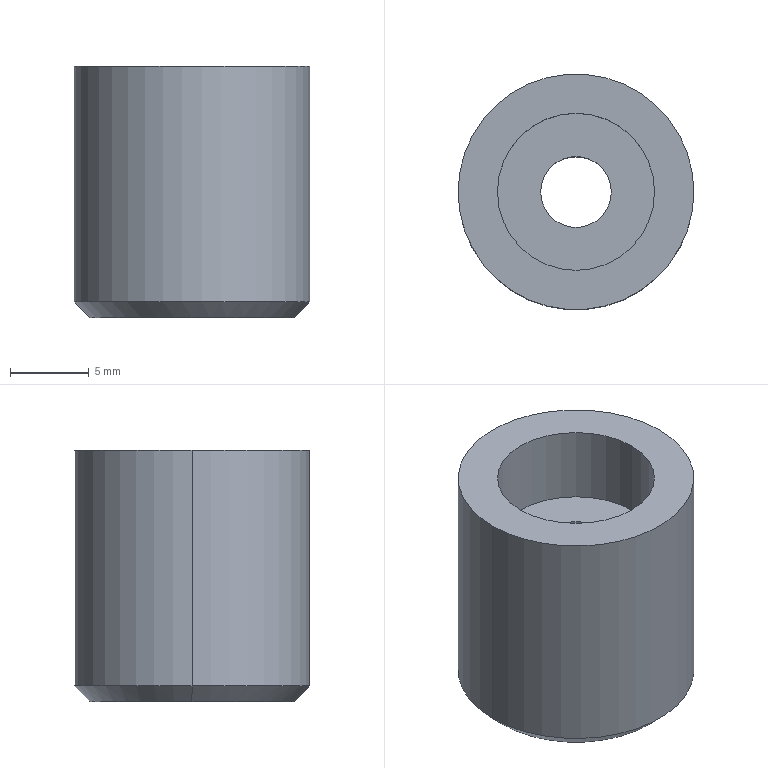Part | STEP file | 2074 Stop shaft 2 | 1 solid | 14 faces | box 15 x 15 x 16 mm | volume 2079 mm3 | cylinder 8 | plane 4 | cone 2 | commonest cylinder face diameters 4.5 x2 8 x2 10 x2 15 x2
STEP:
#1=CARTESIAN_POINT('',(0.,0.,0.));
#2=DIRECTION('',(0.,0.,1.));
#3=DIRECTION('',(1.,0.,0.));
#4=AXIS2_PLACEMENT_3D('',#1,#2,#3);
#5=CARTESIAN_POINT('',(-6.5,0.,0.));
#6=VERTEX_POINT('',#5);
#7=CARTESIAN_POINT('',(6.5,0.,0.));
#8=VERTEX_POINT('',#7);
#9=CARTESIAN_POINT('',(0.,0.,0.));
#10=DIRECTION('',(0.,0.,-1.));
#11=DIRECTION('',(1.,0.,0.));
#12=AXIS2_PLACEMENT_3D('',#9,#10,#11);
#13=CIRCLE('',#12,6.5);
#14=CARTESIAN_POINT('',(0.,0.,1.));
#15=DIRECTION('',(0.,0.,1.));
#16=DIRECTION('',(1.,0.,0.));
#17=AXIS2_PLACEMENT_3D('',#14,#15,#16);
#18=CONICAL_SURFACE('',#17,7.5,0.7854);
#19=CARTESIAN_POINT('',(6.283,-1.));
#20=DIRECTION('',(-1.,0.));
#21=VECTOR('',#20,1.);
#22=LINE('',#19,#21);
#23=(GEOMETRIC_REPRESENTATION_CONTEXT(2)PARAMETRIC_REPRESENTATION_CONTEXT()REPRESENTATION_CONTEXT('',''));
#24=DEFINITIONAL_REPRESENTATION('',(#22),#23);
#25=PCURVE('',#18,#24);
#26=CARTESIAN_POINT('',(0.,0.,0.));
#27=DIRECTION('',(0.,0.,1.));
#28=DIRECTION('',(1.,0.,0.));
#29=AXIS2_PLACEMENT_3D('',#26,#27,#28);
#30=PLANE('',#29);
#31=CARTESIAN_POINT('',(6.5,0.));
#32=CARTESIAN_POINT('',(6.5,-11.258));
#33=CARTESIAN_POINT('',(-3.25,-5.629));
#34=CARTESIAN_POINT('',(-13.,0.));
#35=CARTESIAN_POINT('',(-3.25,5.629));
#36=CARTESIAN_POINT('',(6.5,11.258));
#37=CARTESIAN_POINT('',(6.5,0.));
#38=(BOUNDED_CURVE()B_SPLINE_CURVE(2,(#31,#32,#33,#34,#35,#36,#37),.UNSPECIFIED.,.T.,.F.)B_SPLINE_CURVE_WITH_KNOTS((1,2,2,2,2,1),(-2.094,0.,2.094,4.189,6.283,8.378),.UNSPECIFIED.)CURVE()GEOMETRIC_REPRESENTATION_ITEM()RATIONAL_B_SPLINE_CURVE((1.,0.5,1.,0.5,1.,0.5,1.))REPRESENTATION_ITEM(''));
#39=(GEOMETRIC_REPRESENTATION_CONTEXT(2)PARAMETRIC_REPRESENTATION_CONTEXT()REPRESENTATION_CONTEXT('',''));
#40=DEFINITIONAL_REPRESENTATION('',(#38),#39);
#41=PCURVE('',#30,#40);
#42=SURFACE_CURVE('',#13,(#25,#41),.PCURVE_S1.);
#43=EDGE_CURVE('',#6,#8,#42,.T.);
#44=ORIENTED_EDGE('',*,*,#43,.F.);
#45=CARTESIAN_POINT('',(-7.5,0.,1.));
#46=VERTEX_POINT('',#45);
#47=CARTESIAN_POINT('',(-7.5,0.,1.));
#48=DIRECTION('',(-0.7071,0.,0.7071));
#49=VECTOR('',#48,1.);
#50=LINE('',#47,#49);
#51=CARTESIAN_POINT('',(3.142,0.));
#52=DIRECTION('',(0.,1.));
#53=VECTOR('',#52,1.);
#54=LINE('',#51,#53);
#55=(GEOMETRIC_REPRESENTATION_CONTEXT(2)PARAMETRIC_REPRESENTATION_CONTEXT()REPRESENTATION_CONTEXT('',''));
#56=DEFINITIONAL_REPRESENTATION('',(#54),#55);
#57=PCURVE('',#18,#56);
#58=CARTESIAN_POINT('',(0.,0.,1.));
#59=DIRECTION('',(0.,0.,1.));
#60=DIRECTION('',(1.,0.,0.));
#61=AXIS2_PLACEMENT_3D('',#58,#59,#60);
#62=CONICAL_SURFACE('',#61,7.5,0.7854);
#63=CARTESIAN_POINT('',(3.142,0.));
#64=DIRECTION('',(0.,1.));
#65=VECTOR('',#64,1.);
#66=LINE('',#63,#65);
#67=(GEOMETRIC_REPRESENTATION_CONTEXT(2)PARAMETRIC_REPRESENTATION_CONTEXT()REPRESENTATION_CONTEXT('',''));
#68=DEFINITIONAL_REPRESENTATION('',(#66),#67);
#69=PCURVE('',#62,#68);
#70=SURFACE_CURVE('',#50,(#57,#69),.PCURVE_S1.);
#71=EDGE_CURVE('',#6,#46,#70,.T.);
#72=ORIENTED_EDGE('',*,*,#71,.T.);
#73=CARTESIAN_POINT('',(7.5,0.,1.));
#74=VERTEX_POINT('',#73);
#75=CARTESIAN_POINT('',(0.,0.,1.));
#76=DIRECTION('',(0.,0.,1.));
#77=DIRECTION('',(1.,0.,0.));
#78=AXIS2_PLACEMENT_3D('',#75,#76,#77);
#79=CIRCLE('',#78,7.5);
#80=CARTESIAN_POINT('',(0.,0.));
#81=DIRECTION('',(1.,0.));
#82=VECTOR('',#81,1.);
#83=LINE('',#80,#82);
#84=(GEOMETRIC_REPRESENTATION_CONTEXT(2)PARAMETRIC_REPRESENTATION_CONTEXT()REPRESENTATION_CONTEXT('',''));
#85=DEFINITIONAL_REPRESENTATION('',(#83),#84);
#86=PCURVE('',#18,#85);
#87=CARTESIAN_POINT('',(0.,0.,16.));
#88=DIRECTION('',(0.,0.,-1.));
#89=DIRECTION('',(-1.,0.,0.));
#90=AXIS2_PLACEMENT_3D('',#87,#88,#89);
#91=CYLINDRICAL_SURFACE('',#90,7.5);
#92=CARTESIAN_POINT('',(3.142,15.));
#93=DIRECTION('',(-1.,0.));
#94=VECTOR('',#93,1.);
#95=LINE('',#92,#94);
#96=(GEOMETRIC_REPRESENTATION_CONTEXT(2)PARAMETRIC_REPRESENTATION_CONTEXT()REPRESENTATION_CONTEXT('',''));
#97=DEFINITIONAL_REPRESENTATION('',(#95),#96);
#98=PCURVE('',#91,#97);
#99=SURFACE_CURVE('',#79,(#86,#98),.PCURVE_S1.);
#100=EDGE_CURVE('',#74,#46,#99,.T.);
#101=ORIENTED_EDGE('',*,*,#100,.F.);
#102=CARTESIAN_POINT('',(7.5,0.,1.));
#103=DIRECTION('',(0.7071,0.,0.7071));
#104=VECTOR('',#103,1.);
#105=LINE('',#102,#104);
#106=CARTESIAN_POINT('',(0.,0.));
#107=DIRECTION('',(0.,1.));
#108=VECTOR('',#107,1.);
#109=LINE('',#106,#108);
#110=(GEOMETRIC_REPRESENTATION_CONTEXT(2)PARAMETRIC_REPRESENTATION_CONTEXT()REPRESENTATION_CONTEXT('',''));
#111=DEFINITIONAL_REPRESENTATION('',(#109),#110);
#112=PCURVE('',#18,#111);
#113=CARTESIAN_POINT('',(6.283,0.));
#114=DIRECTION('',(0.,1.));
#115=VECTOR('',#114,1.);
#116=LINE('',#113,#115);
#117=(GEOMETRIC_REPRESENTATION_CONTEXT(2)PARAMETRIC_REPRESENTATION_CONTEXT()REPRESENTATION_CONTEXT('',''));
#118=DEFINITIONAL_REPRESENTATION('',(#116),#117);
#119=PCURVE('',#62,#118);
#120=SURFACE_CURVE('',#105,(#112,#119),.PCURVE_S1.);
#121=EDGE_CURVE('',#8,#74,#120,.T.);
#122=ORIENTED_EDGE('',*,*,#121,.F.);
#123=EDGE_LOOP('',(#44,#72,#101,#122));
#124=FACE_BOUND('',#123,.T.);
#125=ADVANCED_FACE('',(#124),#18,.T.);
#126=CARTESIAN_POINT('',(5.,0.,11.));
#127=VERTEX_POINT('',#126);
#128=CARTESIAN_POINT('',(5.,0.,16.));
#129=VERTEX_POINT('',#128);
#130=CARTESIAN_POINT('',(5.,0.,11.));
#131=DIRECTION('',(0.,0.,1.));
#132=VECTOR('',#131,1.);
#133=LINE('',#130,#132);
#134=CARTESIAN_POINT('',(0.,0.,11.));
#135=DIRECTION('',(0.,0.,1.));
#136=DIRECTION('',(1.,0.,0.));
#137=AXIS2_PLACEMENT_3D('',#134,#135,#136);
#138=CYLINDRICAL_SURFACE('',#137,5.);
#139=CARTESIAN_POINT('',(6.283,0.));
#140=DIRECTION('',(0.,1.));
#141=VECTOR('',#140,1.);
#142=LINE('',#139,#141);
#143=(GEOMETRIC_REPRESENTATION_CONTEXT(2)PARAMETRIC_REPRESENTATION_CONTEXT()REPRESENTATION_CONTEXT('',''));
#144=DEFINITIONAL_REPRESENTATION('',(#142),#143);
#145=PCURVE('',#138,#144);
#146=CARTESIAN_POINT('',(0.,0.,11.));
#147=DIRECTION('',(0.,0.,1.));
#148=DIRECTION('',(1.,0.,0.));
#149=AXIS2_PLACEMENT_3D('',#146,#147,#148);
#150=CYLINDRICAL_SURFACE('',#149,5.);
#151=CARTESIAN_POINT('',(0.,0.));
#152=DIRECTION('',(0.,1.));
#153=VECTOR('',#152,1.);
#154=LINE('',#151,#153);
#155=(GEOMETRIC_REPRESENTATION_CONTEXT(2)PARAMETRIC_REPRESENTATION_CONTEXT()REPRESENTATION_CONTEXT('',''));
#156=DEFINITIONAL_REPRESENTATION('',(#154),#155);
#157=PCURVE('',#150,#156);
#158=SURFACE_CURVE('',#133,(#145,#157),.PCURVE_S1.);
#159=EDGE_CURVE('',#127,#129,#158,.T.);
#160=ORIENTED_EDGE('',*,*,#159,.T.);
#161=CARTESIAN_POINT('',(-5.,0.,16.));
#162=VERTEX_POINT('',#161);
#163=CARTESIAN_POINT('',(0.,0.,16.));
#164=DIRECTION('',(0.,0.,1.));
#165=DIRECTION('',(1.,0.,0.));
#166=AXIS2_PLACEMENT_3D('',#163,#164,#165);
#167=CIRCLE('',#166,5.);
#168=CARTESIAN_POINT('',(0.,5.));
#169=DIRECTION('',(1.,0.));
#170=VECTOR('',#169,1.);
#171=LINE('',#168,#170);
#172=(GEOMETRIC_REPRESENTATION_CONTEXT(2)PARAMETRIC_REPRESENTATION_CONTEXT()REPRESENTATION_CONTEXT('',''));
#173=DEFINITIONAL_REPRESENTATION('',(#171),#172);
#174=PCURVE('',#138,#173);
#175=CARTESIAN_POINT('',(0.,0.,16.));
#176=DIRECTION('',(0.,0.,1.));
#177=DIRECTION('',(1.,0.,0.));
#178=AXIS2_PLACEMENT_3D('',#175,#176,#177);
#179=PLANE('',#178);
#180=CARTESIAN_POINT('',(0.,0.));
#181=DIRECTION('',(1.,0.));
#182=AXIS2_PLACEMENT_2D('',#180,#181);
#183=CIRCLE('',#182,5.);
#184=(GEOMETRIC_REPRESENTATION_CONTEXT(2)PARAMETRIC_REPRESENTATION_CONTEXT()REPRESENTATION_CONTEXT('',''));
#185=DEFINITIONAL_REPRESENTATION('',(#183),#184);
#186=PCURVE('',#179,#185);
#187=SURFACE_CURVE('',#167,(#174,#186),.PCURVE_S1.);
#188=EDGE_CURVE('',#162,#129,#187,.T.);
#189=ORIENTED_EDGE('',*,*,#188,.F.);
#190=CARTESIAN_POINT('',(-5.,0.,11.));
#191=VERTEX_POINT('',#190);
#192=CARTESIAN_POINT('',(-5.,0.,11.));
#193=DIRECTION('',(0.,0.,1.));
#194=VECTOR('',#193,1.);
#195=LINE('',#192,#194);
#196=CARTESIAN_POINT('',(3.142,0.));
#197=DIRECTION('',(0.,1.));
#198=VECTOR('',#197,1.);
#199=LINE('',#196,#198);
#200=(GEOMETRIC_REPRESENTATION_CONTEXT(2)PARAMETRIC_REPRESENTATION_CONTEXT()REPRESENTATION_CONTEXT('',''));
#201=DEFINITIONAL_REPRESENTATION('',(#199),#200);
#202=PCURVE('',#138,#201);
#203=CARTESIAN_POINT('',(3.142,0.));
#204=DIRECTION('',(0.,1.));
#205=VECTOR('',#204,1.);
#206=LINE('',#203,#205);
#207=(GEOMETRIC_REPRESENTATION_CONTEXT(2)PARAMETRIC_REPRESENTATION_CONTEXT()REPRESENTATION_CONTEXT('',''));
#208=DEFINITIONAL_REPRESENTATION('',(#206),#207);
#209=PCURVE('',#150,#208);
#210=SURFACE_CURVE('',#195,(#202,#209),.PCURVE_S1.);
#211=EDGE_CURVE('',#191,#162,#210,.T.);
#212=ORIENTED_EDGE('',*,*,#211,.F.);
#213=CARTESIAN_POINT('',(0.,0.,11.));
#214=DIRECTION('',(0.,0.,1.));
#215=DIRECTION('',(1.,0.,0.));
#216=AXIS2_PLACEMENT_3D('',#213,#214,#215);
#217=CIRCLE('',#216,5.);
#218=CARTESIAN_POINT('',(0.,0.));
#219=DIRECTION('',(1.,0.));
#220=VECTOR('',#219,1.);
#221=LINE('',#218,#220);
#222=(GEOMETRIC_REPRESENTATION_CONTEXT(2)PARAMETRIC_REPRESENTATION_CONTEXT()REPRESENTATION_CONTEXT('',''));
#223=DEFINITIONAL_REPRESENTATION('',(#221),#222);
#224=PCURVE('',#138,#223);
#225=CARTESIAN_POINT('',(0.,0.,11.));
#226=DIRECTION('',(0.,0.,1.));
#227=DIRECTION('',(1.,0.,0.));
#228=AXIS2_PLACEMENT_3D('',#225,#226,#227);
#229=PLANE('',#228);
#230=CARTESIAN_POINT('',(0.,0.));
#231=DIRECTION('',(1.,0.));
#232=AXIS2_PLACEMENT_2D('',#230,#231);
#233=CIRCLE('',#232,5.);
#234=(GEOMETRIC_REPRESENTATION_CONTEXT(2)PARAMETRIC_REPRESENTATION_CONTEXT()REPRESENTATION_CONTEXT('',''));
#235=DEFINITIONAL_REPRESENTATION('',(#233),#234);
#236=PCURVE('',#229,#235);
#237=SURFACE_CURVE('',#217,(#224,#236),.PCURVE_S1.);
#238=EDGE_CURVE('',#191,#127,#237,.T.);
#239=ORIENTED_EDGE('',*,*,#238,.T.);
#240=EDGE_LOOP('',(#160,#189,#212,#239));
#241=FACE_BOUND('',#240,.F.);
#242=ADVANCED_FACE('',(#241),#138,.F.);
#243=CARTESIAN_POINT('',(-4.,0.,4.6));
#244=VERTEX_POINT('',#243);
#245=CARTESIAN_POINT('',(-4.,0.,0.));
#246=VERTEX_POINT('',#245);
#247=CARTESIAN_POINT('',(-4.,0.,0.));
#248=DIRECTION('',(0.,0.,-1.));
#249=VECTOR('',#248,1.);
#250=LINE('',#247,#249);
#251=CARTESIAN_POINT('',(0.,0.,0.));
#252=DIRECTION('',(0.,0.,-1.));
#253=DIRECTION('',(-1.,0.,0.));
#254=AXIS2_PLACEMENT_3D('',#251,#252,#253);
#255=CYLINDRICAL_SURFACE('',#254,4.);
#256=CARTESIAN_POINT('',(6.283,0.));
#257=DIRECTION('',(0.,1.));
#258=VECTOR('',#257,1.);
#259=LINE('',#256,#258);
#260=(GEOMETRIC_REPRESENTATION_CONTEXT(2)PARAMETRIC_REPRESENTATION_CONTEXT()REPRESENTATION_CONTEXT('',''));
#261=DEFINITIONAL_REPRESENTATION('',(#259),#260);
#262=PCURVE('',#255,#261);
#263=CARTESIAN_POINT('',(0.,0.,0.));
#264=DIRECTION('',(0.,0.,-1.));
#265=DIRECTION('',(-1.,0.,0.));
#266=AXIS2_PLACEMENT_3D('',#263,#264,#265);
#267=CYLINDRICAL_SURFACE('',#266,4.);
#268=CARTESIAN_POINT('',(0.,0.));
#269=DIRECTION('',(0.,1.));
#270=VECTOR('',#269,1.);
#271=LINE('',#268,#270);
#272=(GEOMETRIC_REPRESENTATION_CONTEXT(2)PARAMETRIC_REPRESENTATION_CONTEXT()REPRESENTATION_CONTEXT('',''));
#273=DEFINITIONAL_REPRESENTATION('',(#271),#272);
#274=PCURVE('',#267,#273);
#275=SURFACE_CURVE('',#250,(#262,#274),.PCURVE_S1.);
#276=EDGE_CURVE('',#244,#246,#275,.T.);
#277=ORIENTED_EDGE('',*,*,#276,.T.);
#278=CARTESIAN_POINT('',(4.,0.,0.));
#279=VERTEX_POINT('',#278);
#280=CARTESIAN_POINT('',(0.,0.,0.));
#281=DIRECTION('',(0.,0.,-1.));
#282=DIRECTION('',(-1.,0.,0.));
#283=AXIS2_PLACEMENT_3D('',#280,#281,#282);
#284=CIRCLE('',#283,4.);
#285=CARTESIAN_POINT('',(0.,0.));
#286=DIRECTION('',(1.,0.));
#287=VECTOR('',#286,1.);
#288=LINE('',#285,#287);
#289=(GEOMETRIC_REPRESENTATION_CONTEXT(2)PARAMETRIC_REPRESENTATION_CONTEXT()REPRESENTATION_CONTEXT('',''));
#290=DEFINITIONAL_REPRESENTATION('',(#288),#289);
#291=PCURVE('',#255,#290);
#292=CARTESIAN_POINT('',(-4.,0.));
#293=CARTESIAN_POINT('',(-4.,6.928));
#294=CARTESIAN_POINT('',(2.,3.464));
#295=CARTESIAN_POINT('',(8.,0.));
#296=CARTESIAN_POINT('',(2.,-3.464));
#297=CARTESIAN_POINT('',(-4.,-6.928));
#298=CARTESIAN_POINT('',(-4.,0.));
#299=(BOUNDED_CURVE()B_SPLINE_CURVE(2,(#292,#293,#294,#295,#296,#297,#298),.UNSPECIFIED.,.T.,.F.)B_SPLINE_CURVE_WITH_KNOTS((1,2,2,2,2,1),(-2.094,0.,2.094,4.189,6.283,8.378),.UNSPECIFIED.)CURVE()GEOMETRIC_REPRESENTATION_ITEM()RATIONAL_B_SPLINE_CURVE((1.,0.5,1.,0.5,1.,0.5,1.))REPRESENTATION_ITEM(''));
#300=(GEOMETRIC_REPRESENTATION_CONTEXT(2)PARAMETRIC_REPRESENTATION_CONTEXT()REPRESENTATION_CONTEXT('',''));
#301=DEFINITIONAL_REPRESENTATION('',(#299),#300);
#302=PCURVE('',#30,#301);
#303=SURFACE_CURVE('',#284,(#291,#302),.PCURVE_S1.);
#304=EDGE_CURVE('',#279,#246,#303,.T.);
#305=ORIENTED_EDGE('',*,*,#304,.F.);
#306=CARTESIAN_POINT('',(4.,0.,4.6));
#307=VERTEX_POINT('',#306);
#308=CARTESIAN_POINT('',(4.,0.,0.));
#309=DIRECTION('',(0.,0.,-1.));
#310=VECTOR('',#309,1.);
#311=LINE('',#308,#310);
#312=CARTESIAN_POINT('',(3.142,0.));
#313=DIRECTION('',(0.,1.));
#314=VECTOR('',#313,1.);
#315=LINE('',#312,#314);
#316=(GEOMETRIC_REPRESENTATION_CONTEXT(2)PARAMETRIC_REPRESENTATION_CONTEXT()REPRESENTATION_CONTEXT('',''));
#317=DEFINITIONAL_REPRESENTATION('',(#315),#316);
#318=PCURVE('',#255,#317);
#319=CARTESIAN_POINT('',(3.142,0.));
#320=DIRECTION('',(0.,1.));
#321=VECTOR('',#320,1.);
#322=LINE('',#319,#321);
#323=(GEOMETRIC_REPRESENTATION_CONTEXT(2)PARAMETRIC_REPRESENTATION_CONTEXT()REPRESENTATION_CONTEXT('',''));
#324=DEFINITIONAL_REPRESENTATION('',(#322),#323);
#325=PCURVE('',#267,#324);
#326=SURFACE_CURVE('',#311,(#318,#325),.PCURVE_S1.);
#327=EDGE_CURVE('',#307,#279,#326,.T.);
#328=ORIENTED_EDGE('',*,*,#327,.F.);
#329=CARTESIAN_POINT('',(0.,0.,4.6));
#330=DIRECTION('',(0.,0.,-1.));
#331=DIRECTION('',(-1.,0.,0.));
#332=AXIS2_PLACEMENT_3D('',#329,#330,#331);
#333=CIRCLE('',#332,4.);
#334=CARTESIAN_POINT('',(0.,-4.6));
#335=DIRECTION('',(1.,0.));
#336=VECTOR('',#335,1.);
#337=LINE('',#334,#336);
#338=(GEOMETRIC_REPRESENTATION_CONTEXT(2)PARAMETRIC_REPRESENTATION_CONTEXT()REPRESENTATION_CONTEXT('',''));
#339=DEFINITIONAL_REPRESENTATION('',(#337),#338);
#340=PCURVE('',#255,#339);
#341=CARTESIAN_POINT('',(2.25,0.,4.6));
#342=DIRECTION('',(0.,0.,1.));
#343=DIRECTION('',(1.,0.,0.));
#344=AXIS2_PLACEMENT_3D('',#341,#342,#343);
#345=PLANE('',#344);
#346=CARTESIAN_POINT('',(-6.25,0.));
#347=CARTESIAN_POINT('',(-6.25,6.928));
#348=CARTESIAN_POINT('',(-0.25,3.464));
#349=CARTESIAN_POINT('',(5.75,0.));
#350=CARTESIAN_POINT('',(-0.25,-3.464));
#351=CARTESIAN_POINT('',(-6.25,-6.928));
#352=CARTESIAN_POINT('',(-6.25,0.));
#353=(BOUNDED_CURVE()B_SPLINE_CURVE(2,(#346,#347,#348,#349,#350,#351,#352),.UNSPECIFIED.,.T.,.F.)B_SPLINE_CURVE_WITH_KNOTS((1,2,2,2,2,1),(-2.094,0.,2.094,4.189,6.283,8.378),.UNSPECIFIED.)CURVE()GEOMETRIC_REPRESENTATION_ITEM()RATIONAL_B_SPLINE_CURVE((1.,0.5,1.,0.5,1.,0.5,1.))REPRESENTATION_ITEM(''));
#354=(GEOMETRIC_REPRESENTATION_CONTEXT(2)PARAMETRIC_REPRESENTATION_CONTEXT()REPRESENTATION_CONTEXT('',''));
#355=DEFINITIONAL_REPRESENTATION('',(#353),#354);
#356=PCURVE('',#345,#355);
#357=SURFACE_CURVE('',#333,(#340,#356),.PCURVE_S1.);
#358=EDGE_CURVE('',#307,#244,#357,.T.);
#359=ORIENTED_EDGE('',*,*,#358,.T.);
#360=EDGE_LOOP('',(#277,#305,#328,#359));
#361=FACE_BOUND('',#360,.F.);
#362=ADVANCED_FACE('',(#361),#255,.F.);
#363=CARTESIAN_POINT('',(7.5,0.,16.));
#364=VERTEX_POINT('',#363);
#365=CARTESIAN_POINT('',(-7.5,0.,16.));
#366=VERTEX_POINT('',#365);
#367=CARTESIAN_POINT('',(0.,0.,16.));
#368=DIRECTION('',(0.,0.,1.));
#369=DIRECTION('',(1.,0.,0.));
#370=AXIS2_PLACEMENT_3D('',#367,#368,#369);
#371=CIRCLE('',#370,7.5);
#372=CARTESIAN_POINT('',(3.142,0.));
#373=DIRECTION('',(-1.,0.));
#374=VECTOR('',#373,1.);
#375=LINE('',#372,#374);
#376=(GEOMETRIC_REPRESENTATION_CONTEXT(2)PARAMETRIC_REPRESENTATION_CONTEXT()REPRESENTATION_CONTEXT('',''));
#377=DEFINITIONAL_REPRESENTATION('',(#375),#376);
#378=PCURVE('',#91,#377);
#379=CARTESIAN_POINT('',(0.,0.));
#380=DIRECTION('',(1.,0.));
#381=AXIS2_PLACEMENT_2D('',#379,#380);
#382=CIRCLE('',#381,7.5);
#383=(GEOMETRIC_REPRESENTATION_CONTEXT(2)PARAMETRIC_REPRESENTATION_CONTEXT()REPRESENTATION_CONTEXT('',''));
#384=DEFINITIONAL_REPRESENTATION('',(#382),#383);
#385=PCURVE('',#179,#384);
#386=SURFACE_CURVE('',#371,(#378,#385),.PCURVE_S1.);
#387=EDGE_CURVE('',#364,#366,#386,.T.);
#388=ORIENTED_EDGE('',*,*,#387,.F.);
#389=CARTESIAN_POINT('',(7.5,0.,16.));
#390=DIRECTION('',(0.,0.,-1.));
#391=VECTOR('',#390,1.);
#392=LINE('',#389,#391);
#393=CARTESIAN_POINT('',(3.142,0.));
#394=DIRECTION('',(0.,1.));
#395=VECTOR('',#394,1.);
#396=LINE('',#393,#395);
#397=(GEOMETRIC_REPRESENTATION_CONTEXT(2)PARAMETRIC_REPRESENTATION_CONTEXT()REPRESENTATION_CONTEXT('',''));
#398=DEFINITIONAL_REPRESENTATION('',(#396),#397);
#399=PCURVE('',#91,#398);
#400=CARTESIAN_POINT('',(0.,0.,16.));
#401=DIRECTION('',(0.,0.,-1.));
#402=DIRECTION('',(-1.,0.,0.));
#403=AXIS2_PLACEMENT_3D('',#400,#401,#402);
#404=CYLINDRICAL_SURFACE('',#403,7.5);
#405=CARTESIAN_POINT('',(3.142,0.));
#406=DIRECTION('',(0.,1.));
#407=VECTOR('',#406,1.);
#408=LINE('',#405,#407);
#409=(GEOMETRIC_REPRESENTATION_CONTEXT(2)PARAMETRIC_REPRESENTATION_CONTEXT()REPRESENTATION_CONTEXT('',''));
#410=DEFINITIONAL_REPRESENTATION('',(#408),#409);
#411=PCURVE('',#404,#410);
#412=SURFACE_CURVE('',#392,(#399,#411),.PCURVE_S1.);
#413=EDGE_CURVE('',#364,#74,#412,.T.);
#414=ORIENTED_EDGE('',*,*,#413,.T.);
#415=ORIENTED_EDGE('',*,*,#100,.T.);
#416=CARTESIAN_POINT('',(-7.5,0.,16.));
#417=DIRECTION('',(0.,0.,-1.));
#418=VECTOR('',#417,1.);
#419=LINE('',#416,#418);
#420=CARTESIAN_POINT('',(0.,0.));
#421=DIRECTION('',(0.,1.));
#422=VECTOR('',#421,1.);
#423=LINE('',#420,#422);
#424=(GEOMETRIC_REPRESENTATION_CONTEXT(2)PARAMETRIC_REPRESENTATION_CONTEXT()REPRESENTATION_CONTEXT('',''));
#425=DEFINITIONAL_REPRESENTATION('',(#423),#424);
#426=PCURVE('',#91,#425);
#427=CARTESIAN_POINT('',(6.283,0.));
#428=DIRECTION('',(0.,1.));
#429=VECTOR('',#428,1.);
#430=LINE('',#427,#429);
#431=(GEOMETRIC_REPRESENTATION_CONTEXT(2)PARAMETRIC_REPRESENTATION_CONTEXT()REPRESENTATION_CONTEXT('',''));
#432=DEFINITIONAL_REPRESENTATION('',(#430),#431);
#433=PCURVE('',#404,#432);
#434=SURFACE_CURVE('',#419,(#426,#433),.PCURVE_S1.);
#435=EDGE_CURVE('',#366,#46,#434,.T.);
#436=ORIENTED_EDGE('',*,*,#435,.F.);
#437=EDGE_LOOP('',(#388,#414,#415,#436));
#438=FACE_BOUND('',#437,.T.);
#439=ADVANCED_FACE('',(#438),#91,.T.);
#440=CARTESIAN_POINT('',(-2.25,0.,11.));
#441=VERTEX_POINT('',#440);
#442=CARTESIAN_POINT('',(-2.25,0.,4.6));
#443=VERTEX_POINT('',#442);
#444=CARTESIAN_POINT('',(-2.25,0.,0.));
#445=DIRECTION('',(0.,0.,-1.));
#446=VECTOR('',#445,1.);
#447=LINE('',#444,#446);
#448=CARTESIAN_POINT('',(0.,0.,0.));
#449=DIRECTION('',(0.,0.,-1.));
#450=DIRECTION('',(-1.,0.,0.));
#451=AXIS2_PLACEMENT_3D('',#448,#449,#450);
#452=CYLINDRICAL_SURFACE('',#451,2.25);
#453=CARTESIAN_POINT('',(6.283,0.));
#454=DIRECTION('',(0.,1.));
#455=VECTOR('',#454,1.);
#456=LINE('',#453,#455);
#457=(GEOMETRIC_REPRESENTATION_CONTEXT(2)PARAMETRIC_REPRESENTATION_CONTEXT()REPRESENTATION_CONTEXT('',''));
#458=DEFINITIONAL_REPRESENTATION('',(#456),#457);
#459=PCURVE('',#452,#458);
#460=CARTESIAN_POINT('',(0.,0.,0.));
#461=DIRECTION('',(0.,0.,-1.));
#462=DIRECTION('',(-1.,0.,0.));
#463=AXIS2_PLACEMENT_3D('',#460,#461,#462);
#464=CYLINDRICAL_SURFACE('',#463,2.25);
#465=CARTESIAN_POINT('',(0.,0.));
#466=DIRECTION('',(0.,1.));
#467=VECTOR('',#466,1.);
#468=LINE('',#465,#467);
#469=(GEOMETRIC_REPRESENTATION_CONTEXT(2)PARAMETRIC_REPRESENTATION_CONTEXT()REPRESENTATION_CONTEXT('',''));
#470=DEFINITIONAL_REPRESENTATION('',(#468),#469);
#471=PCURVE('',#464,#470);
#472=SURFACE_CURVE('',#447,(#459,#471),.PCURVE_S1.);
#473=EDGE_CURVE('',#441,#443,#472,.T.);
#474=ORIENTED_EDGE('',*,*,#473,.T.);
#475=CARTESIAN_POINT('',(2.25,0.,4.6));
#476=VERTEX_POINT('',#475);
#477=CARTESIAN_POINT('',(0.,0.,4.6));
#478=DIRECTION('',(0.,0.,-1.));
#479=DIRECTION('',(-1.,0.,0.));
#480=AXIS2_PLACEMENT_3D('',#477,#478,#479);
#481=CIRCLE('',#480,2.25);
#482=CARTESIAN_POINT('',(0.,-4.6));
#483=DIRECTION('',(1.,0.));
#484=VECTOR('',#483,1.);
#485=LINE('',#482,#484);
#486=(GEOMETRIC_REPRESENTATION_CONTEXT(2)PARAMETRIC_REPRESENTATION_CONTEXT()REPRESENTATION_CONTEXT('',''));
#487=DEFINITIONAL_REPRESENTATION('',(#485),#486);
#488=PCURVE('',#452,#487);
#489=CARTESIAN_POINT('',(-4.5,0.));
#490=CARTESIAN_POINT('',(-4.5,3.897));
#491=CARTESIAN_POINT('',(-1.125,1.949));
#492=CARTESIAN_POINT('',(2.25,0.));
#493=CARTESIAN_POINT('',(-1.125,-1.949));
#494=CARTESIAN_POINT('',(-4.5,-3.897));
#495=CARTESIAN_POINT('',(-4.5,0.));
#496=(BOUNDED_CURVE()B_SPLINE_CURVE(2,(#489,#490,#491,#492,#493,#494,#495),.UNSPECIFIED.,.T.,.F.)B_SPLINE_CURVE_WITH_KNOTS((1,2,2,2,2,1),(-2.094,0.,2.094,4.189,6.283,8.378),.UNSPECIFIED.)CURVE()GEOMETRIC_REPRESENTATION_ITEM()RATIONAL_B_SPLINE_CURVE((1.,0.5,1.,0.5,1.,0.5,1.))REPRESENTATION_ITEM(''));
#497=(GEOMETRIC_REPRESENTATION_CONTEXT(2)PARAMETRIC_REPRESENTATION_CONTEXT()REPRESENTATION_CONTEXT('',''));
#498=DEFINITIONAL_REPRESENTATION('',(#496),#497);
#499=PCURVE('',#345,#498);
#500=SURFACE_CURVE('',#481,(#488,#499),.PCURVE_S1.);
#501=EDGE_CURVE('',#476,#443,#500,.T.);
#502=ORIENTED_EDGE('',*,*,#501,.F.);
#503=CARTESIAN_POINT('',(2.25,0.,11.));
#504=VERTEX_POINT('',#503);
#505=CARTESIAN_POINT('',(2.25,0.,0.));
#506=DIRECTION('',(0.,0.,-1.));
#507=VECTOR('',#506,1.);
#508=LINE('',#505,#507);
#509=CARTESIAN_POINT('',(3.142,0.));
#510=DIRECTION('',(0.,1.));
#511=VECTOR('',#510,1.);
#512=LINE('',#509,#511);
#513=(GEOMETRIC_REPRESENTATION_CONTEXT(2)PARAMETRIC_REPRESENTATION_CONTEXT()REPRESENTATION_CONTEXT('',''));
#514=DEFINITIONAL_REPRESENTATION('',(#512),#513);
#515=PCURVE('',#452,#514);
#516=CARTESIAN_POINT('',(3.142,0.));
#517=DIRECTION('',(0.,1.));
#518=VECTOR('',#517,1.);
#519=LINE('',#516,#518);
#520=(GEOMETRIC_REPRESENTATION_CONTEXT(2)PARAMETRIC_REPRESENTATION_CONTEXT()REPRESENTATION_CONTEXT('',''));
#521=DEFINITIONAL_REPRESENTATION('',(#519),#520);
#522=PCURVE('',#464,#521);
#523=SURFACE_CURVE('',#508,(#515,#522),.PCURVE_S1.);
#524=EDGE_CURVE('',#504,#476,#523,.T.);
#525=ORIENTED_EDGE('',*,*,#524,.F.);
#526=CARTESIAN_POINT('',(0.,0.,11.));
#527=DIRECTION('',(0.,0.,-1.));
#528=DIRECTION('',(1.,0.,0.));
#529=AXIS2_PLACEMENT_3D('',#526,#527,#528);
#530=CIRCLE('',#529,2.25);
#531=CARTESIAN_POINT('',(3.142,-11.));
#532=DIRECTION('',(1.,0.));
#533=VECTOR('',#532,1.);
#534=LINE('',#531,#533);
#535=(GEOMETRIC_REPRESENTATION_CONTEXT(2)PARAMETRIC_REPRESENTATION_CONTEXT()REPRESENTATION_CONTEXT('',''));
#536=DEFINITIONAL_REPRESENTATION('',(#534),#535);
#537=PCURVE('',#452,#536);
#538=CARTESIAN_POINT('',(2.25,0.));
#539=CARTESIAN_POINT('',(2.25,-3.897));
#540=CARTESIAN_POINT('',(-1.125,-1.949));
#541=CARTESIAN_POINT('',(-4.5,0.));
#542=CARTESIAN_POINT('',(-1.125,1.949));
#543=CARTESIAN_POINT('',(2.25,3.897));
#544=CARTESIAN_POINT('',(2.25,0.));
#545=(BOUNDED_CURVE()B_SPLINE_CURVE(2,(#538,#539,#540,#541,#542,#543,#544),.UNSPECIFIED.,.T.,.F.)B_SPLINE_CURVE_WITH_KNOTS((1,2,2,2,2,1),(-2.094,0.,2.094,4.189,6.283,8.378),.UNSPECIFIED.)CURVE()GEOMETRIC_REPRESENTATION_ITEM()RATIONAL_B_SPLINE_CURVE((1.,0.5,1.,0.5,1.,0.5,1.))REPRESENTATION_ITEM(''));
#546=(GEOMETRIC_REPRESENTATION_CONTEXT(2)PARAMETRIC_REPRESENTATION_CONTEXT()REPRESENTATION_CONTEXT('',''));
#547=DEFINITIONAL_REPRESENTATION('',(#545),#546);
#548=PCURVE('',#229,#547);
#549=SURFACE_CURVE('',#530,(#537,#548),.PCURVE_S1.);
#550=EDGE_CURVE('',#504,#441,#549,.T.);
#551=ORIENTED_EDGE('',*,*,#550,.T.);
#552=EDGE_LOOP('',(#474,#502,#525,#551));
#553=FACE_BOUND('',#552,.F.);
#554=ADVANCED_FACE('',(#553),#452,.F.);
#555=CARTESIAN_POINT('',(0.,0.,4.6));
#556=DIRECTION('',(0.,0.,-1.));
#557=DIRECTION('',(-1.,0.,0.));
#558=AXIS2_PLACEMENT_3D('',#555,#556,#557);
#559=CIRCLE('',#558,2.25);
#560=CARTESIAN_POINT('',(0.,-4.6));
#561=DIRECTION('',(1.,0.));
#562=VECTOR('',#561,1.);
#563=LINE('',#560,#562);
#564=(GEOMETRIC_REPRESENTATION_CONTEXT(2)PARAMETRIC_REPRESENTATION_CONTEXT()REPRESENTATION_CONTEXT('',''));
#565=DEFINITIONAL_REPRESENTATION('',(#563),#564);
#566=PCURVE('',#464,#565);
#567=CARTESIAN_POINT('',(-4.5,0.));
#568=CARTESIAN_POINT('',(-4.5,3.897));
#569=CARTESIAN_POINT('',(-1.125,1.949));
#570=CARTESIAN_POINT('',(2.25,0.));
#571=CARTESIAN_POINT('',(-1.125,-1.949));
#572=CARTESIAN_POINT('',(-4.5,-3.897));
#573=CARTESIAN_POINT('',(-4.5,0.));
#574=(BOUNDED_CURVE()B_SPLINE_CURVE(2,(#567,#568,#569,#570,#571,#572,#573),.UNSPECIFIED.,.T.,.F.)B_SPLINE_CURVE_WITH_KNOTS((1,2,2,2,2,1),(-2.094,0.,2.094,4.189,6.283,8.378),.UNSPECIFIED.)CURVE()GEOMETRIC_REPRESENTATION_ITEM()RATIONAL_B_SPLINE_CURVE((1.,0.5,1.,0.5,1.,0.5,1.))REPRESENTATION_ITEM(''));
#575=(GEOMETRIC_REPRESENTATION_CONTEXT(2)PARAMETRIC_REPRESENTATION_CONTEXT()REPRESENTATION_CONTEXT('',''));
#576=DEFINITIONAL_REPRESENTATION('',(#574),#575);
#577=PCURVE('',#345,#576);
#578=SURFACE_CURVE('',#559,(#566,#577),.PCURVE_S1.);
#579=EDGE_CURVE('',#443,#476,#578,.T.);
#580=ORIENTED_EDGE('',*,*,#579,.F.);
#581=ORIENTED_EDGE('',*,*,#473,.F.);
#582=CARTESIAN_POINT('',(0.,0.,11.));
#583=DIRECTION('',(0.,0.,-1.));
#584=DIRECTION('',(1.,0.,0.));
#585=AXIS2_PLACEMENT_3D('',#582,#583,#584);
#586=CIRCLE('',#585,2.25);
#587=CARTESIAN_POINT('',(-3.142,-11.));
#588=DIRECTION('',(1.,0.));
#589=VECTOR('',#588,1.);
#590=LINE('',#587,#589);
#591=(GEOMETRIC_REPRESENTATION_CONTEXT(2)PARAMETRIC_REPRESENTATION_CONTEXT()REPRESENTATION_CONTEXT('',''));
#592=DEFINITIONAL_REPRESENTATION('',(#590),#591);
#593=PCURVE('',#464,#592);
#594=CARTESIAN_POINT('',(2.25,0.));
#595=CARTESIAN_POINT('',(2.25,-3.897));
#596=CARTESIAN_POINT('',(-1.125,-1.949));
#597=CARTESIAN_POINT('',(-4.5,0.));
#598=CARTESIAN_POINT('',(-1.125,1.949));
#599=CARTESIAN_POINT('',(2.25,3.897));
#600=CARTESIAN_POINT('',(2.25,0.));
#601=(BOUNDED_CURVE()B_SPLINE_CURVE(2,(#594,#595,#596,#597,#598,#599,#600),.UNSPECIFIED.,.T.,.F.)B_SPLINE_CURVE_WITH_KNOTS((1,2,2,2,2,1),(-2.094,0.,2.094,4.189,6.283,8.378),.UNSPECIFIED.)CURVE()GEOMETRIC_REPRESENTATION_ITEM()RATIONAL_B_SPLINE_CURVE((1.,0.5,1.,0.5,1.,0.5,1.))REPRESENTATION_ITEM(''));
#602=(GEOMETRIC_REPRESENTATION_CONTEXT(2)PARAMETRIC_REPRESENTATION_CONTEXT()REPRESENTATION_CONTEXT('',''));
#603=DEFINITIONAL_REPRESENTATION('',(#601),#602);
#604=PCURVE('',#229,#603);
#605=SURFACE_CURVE('',#586,(#593,#604),.PCURVE_S1.);
#606=EDGE_CURVE('',#441,#504,#605,.T.);
#607=ORIENTED_EDGE('',*,*,#606,.T.);
#608=ORIENTED_EDGE('',*,*,#524,.T.);
#609=EDGE_LOOP('',(#580,#581,#607,#608));
#610=FACE_BOUND('',#609,.F.);
#611=ADVANCED_FACE('',(#610),#464,.F.);
#612=ORIENTED_EDGE('',*,*,#413,.F.);
#613=CARTESIAN_POINT('',(0.,0.,16.));
#614=DIRECTION('',(0.,0.,1.));
#615=DIRECTION('',(1.,0.,0.));
#616=AXIS2_PLACEMENT_3D('',#613,#614,#615);
#617=CIRCLE('',#616,7.5);
#618=CARTESIAN_POINT('',(9.425,0.));
#619=DIRECTION('',(-1.,0.));
#620=VECTOR('',#619,1.);
#621=LINE('',#618,#620);
#622=(GEOMETRIC_REPRESENTATION_CONTEXT(2)PARAMETRIC_REPRESENTATION_CONTEXT()REPRESENTATION_CONTEXT('',''));
#623=DEFINITIONAL_REPRESENTATION('',(#621),#622);
#624=PCURVE('',#404,#623);
#625=CARTESIAN_POINT('',(0.,0.));
#626=DIRECTION('',(1.,0.));
#627=AXIS2_PLACEMENT_2D('',#625,#626);
#628=CIRCLE('',#627,7.5);
#629=(GEOMETRIC_REPRESENTATION_CONTEXT(2)PARAMETRIC_REPRESENTATION_CONTEXT()REPRESENTATION_CONTEXT('',''));
#630=DEFINITIONAL_REPRESENTATION('',(#628),#629);
#631=PCURVE('',#179,#630);
#632=SURFACE_CURVE('',#617,(#624,#631),.PCURVE_S1.);
#633=EDGE_CURVE('',#366,#364,#632,.T.);
#634=ORIENTED_EDGE('',*,*,#633,.F.);
#635=ORIENTED_EDGE('',*,*,#435,.T.);
#636=CARTESIAN_POINT('',(0.,0.,1.));
#637=DIRECTION('',(0.,0.,1.));
#638=DIRECTION('',(1.,0.,0.));
#639=AXIS2_PLACEMENT_3D('',#636,#637,#638);
#640=CIRCLE('',#639,7.5);
#641=CARTESIAN_POINT('',(9.425,15.));
#642=DIRECTION('',(-1.,0.));
#643=VECTOR('',#642,1.);
#644=LINE('',#641,#643);
#645=(GEOMETRIC_REPRESENTATION_CONTEXT(2)PARAMETRIC_REPRESENTATION_CONTEXT()REPRESENTATION_CONTEXT('',''));
#646=DEFINITIONAL_REPRESENTATION('',(#644),#645);
#647=PCURVE('',#404,#646);
#648=CARTESIAN_POINT('',(0.,0.));
#649=DIRECTION('',(1.,0.));
#650=VECTOR('',#649,1.);
#651=LINE('',#648,#650);
#652=(GEOMETRIC_REPRESENTATION_CONTEXT(2)PARAMETRIC_REPRESENTATION_CONTEXT()REPRESENTATION_CONTEXT('',''));
#653=DEFINITIONAL_REPRESENTATION('',(#651),#652);
#654=PCURVE('',#62,#653);
#655=SURFACE_CURVE('',#640,(#647,#654),.PCURVE_S1.);
#656=EDGE_CURVE('',#46,#74,#655,.T.);
#657=ORIENTED_EDGE('',*,*,#656,.T.);
#658=EDGE_LOOP('',(#612,#634,#635,#657));
#659=FACE_BOUND('',#658,.T.);
#660=ADVANCED_FACE('',(#659),#404,.T.);
#661=CARTESIAN_POINT('',(0.,0.,16.));
#662=DIRECTION('',(0.,0.,1.));
#663=DIRECTION('',(1.,0.,0.));
#664=AXIS2_PLACEMENT_3D('',#661,#662,#663);
#665=CIRCLE('',#664,5.);
#666=CARTESIAN_POINT('',(0.,0.));
#667=DIRECTION('',(1.,0.));
#668=AXIS2_PLACEMENT_2D('',#666,#667);
#669=CIRCLE('',#668,5.);
#670=(GEOMETRIC_REPRESENTATION_CONTEXT(2)PARAMETRIC_REPRESENTATION_CONTEXT()REPRESENTATION_CONTEXT('',''));
#671=DEFINITIONAL_REPRESENTATION('',(#669),#670);
#672=PCURVE('',#179,#671);
#673=CARTESIAN_POINT('',(0.,5.));
#674=DIRECTION('',(1.,0.));
#675=VECTOR('',#674,1.);
#676=LINE('',#673,#675);
#677=(GEOMETRIC_REPRESENTATION_CONTEXT(2)PARAMETRIC_REPRESENTATION_CONTEXT()REPRESENTATION_CONTEXT('',''));
#678=DEFINITIONAL_REPRESENTATION('',(#676),#677);
#679=PCURVE('',#150,#678);
#680=SURFACE_CURVE('',#665,(#672,#679),.PCURVE_S1.);
#681=EDGE_CURVE('',#129,#162,#680,.T.);
#682=ORIENTED_EDGE('',*,*,#681,.F.);
#683=ORIENTED_EDGE('',*,*,#188,.F.);
#684=EDGE_LOOP('',(#682,#683));
#685=FACE_BOUND('',#684,.T.);
#686=ORIENTED_EDGE('',*,*,#633,.T.);
#687=ORIENTED_EDGE('',*,*,#387,.T.);
#688=EDGE_LOOP('',(#686,#687));
#689=FACE_BOUND('',#688,.T.);
#690=ADVANCED_FACE('',(#685,#689),#179,.T.);
#691=CARTESIAN_POINT('',(0.,0.,0.));
#692=DIRECTION('',(0.,0.,-1.));
#693=DIRECTION('',(1.,0.,0.));
#694=AXIS2_PLACEMENT_3D('',#691,#692,#693);
#695=CIRCLE('',#694,6.5);
#696=CARTESIAN_POINT('',(6.5,0.));
#697=CARTESIAN_POINT('',(6.5,-11.258));
#698=CARTESIAN_POINT('',(-3.25,-5.629));
#699=CARTESIAN_POINT('',(-13.,0.));
#700=CARTESIAN_POINT('',(-3.25,5.629));
#701=CARTESIAN_POINT('',(6.5,11.258));
#702=CARTESIAN_POINT('',(6.5,0.));
#703=(BOUNDED_CURVE()B_SPLINE_CURVE(2,(#696,#697,#698,#699,#700,#701,#702),.UNSPECIFIED.,.T.,.F.)B_SPLINE_CURVE_WITH_KNOTS((1,2,2,2,2,1),(-2.094,0.,2.094,4.189,6.283,8.378),.UNSPECIFIED.)CURVE()GEOMETRIC_REPRESENTATION_ITEM()RATIONAL_B_SPLINE_CURVE((1.,0.5,1.,0.5,1.,0.5,1.))REPRESENTATION_ITEM(''));
#704=(GEOMETRIC_REPRESENTATION_CONTEXT(2)PARAMETRIC_REPRESENTATION_CONTEXT()REPRESENTATION_CONTEXT('',''));
#705=DEFINITIONAL_REPRESENTATION('',(#703),#704);
#706=PCURVE('',#30,#705);
#707=CARTESIAN_POINT('',(6.283,-1.));
#708=DIRECTION('',(-1.,0.));
#709=VECTOR('',#708,1.);
#710=LINE('',#707,#709);
#711=(GEOMETRIC_REPRESENTATION_CONTEXT(2)PARAMETRIC_REPRESENTATION_CONTEXT()REPRESENTATION_CONTEXT('',''));
#712=DEFINITIONAL_REPRESENTATION('',(#710),#711);
#713=PCURVE('',#62,#712);
#714=SURFACE_CURVE('',#695,(#706,#713),.PCURVE_S1.);
#715=EDGE_CURVE('',#8,#6,#714,.T.);
#716=ORIENTED_EDGE('',*,*,#715,.T.);
#717=ORIENTED_EDGE('',*,*,#43,.T.);
#718=EDGE_LOOP('',(#716,#717));
#719=FACE_BOUND('',#718,.T.);
#720=CARTESIAN_POINT('',(0.,0.,0.));
#721=DIRECTION('',(0.,0.,-1.));
#722=DIRECTION('',(-1.,0.,0.));
#723=AXIS2_PLACEMENT_3D('',#720,#721,#722);
#724=CIRCLE('',#723,4.);
#725=CARTESIAN_POINT('',(-4.,0.));
#726=CARTESIAN_POINT('',(-4.,6.928));
#727=CARTESIAN_POINT('',(2.,3.464));
#728=CARTESIAN_POINT('',(8.,0.));
#729=CARTESIAN_POINT('',(2.,-3.464));
#730=CARTESIAN_POINT('',(-4.,-6.928));
#731=CARTESIAN_POINT('',(-4.,0.));
#732=(BOUNDED_CURVE()B_SPLINE_CURVE(2,(#725,#726,#727,#728,#729,#730,#731),.UNSPECIFIED.,.T.,.F.)B_SPLINE_CURVE_WITH_KNOTS((1,2,2,2,2,1),(-2.094,0.,2.094,4.189,6.283,8.378),.UNSPECIFIED.)CURVE()GEOMETRIC_REPRESENTATION_ITEM()RATIONAL_B_SPLINE_CURVE((1.,0.5,1.,0.5,1.,0.5,1.))REPRESENTATION_ITEM(''));
#733=(GEOMETRIC_REPRESENTATION_CONTEXT(2)PARAMETRIC_REPRESENTATION_CONTEXT()REPRESENTATION_CONTEXT('',''));
#734=DEFINITIONAL_REPRESENTATION('',(#732),#733);
#735=PCURVE('',#30,#734);
#736=CARTESIAN_POINT('',(0.,0.));
#737=DIRECTION('',(1.,0.));
#738=VECTOR('',#737,1.);
#739=LINE('',#736,#738);
#740=(GEOMETRIC_REPRESENTATION_CONTEXT(2)PARAMETRIC_REPRESENTATION_CONTEXT()REPRESENTATION_CONTEXT('',''));
#741=DEFINITIONAL_REPRESENTATION('',(#739),#740);
#742=PCURVE('',#267,#741);
#743=SURFACE_CURVE('',#724,(#735,#742),.PCURVE_S1.);
#744=EDGE_CURVE('',#246,#279,#743,.T.);
#745=ORIENTED_EDGE('',*,*,#744,.F.);
#746=ORIENTED_EDGE('',*,*,#304,.F.);
#747=EDGE_LOOP('',(#745,#746));
#748=FACE_BOUND('',#747,.T.);
#749=ADVANCED_FACE('',(#719,#748),#30,.F.);
#750=ORIENTED_EDGE('',*,*,#579,.F.);
#751=ORIENTED_EDGE('',*,*,#501,.F.);
#752=EDGE_LOOP('',(#750,#751));
#753=FACE_BOUND('',#752,.T.);
#754=CARTESIAN_POINT('',(0.,0.,4.6));
#755=DIRECTION('',(0.,0.,-1.));
#756=DIRECTION('',(-1.,0.,0.));
#757=AXIS2_PLACEMENT_3D('',#754,#755,#756);
#758=CIRCLE('',#757,4.);
#759=CARTESIAN_POINT('',(-6.25,0.));
#760=CARTESIAN_POINT('',(-6.25,6.928));
#761=CARTESIAN_POINT('',(-0.25,3.464));
#762=CARTESIAN_POINT('',(5.75,0.));
#763=CARTESIAN_POINT('',(-0.25,-3.464));
#764=CARTESIAN_POINT('',(-6.25,-6.928));
#765=CARTESIAN_POINT('',(-6.25,0.));
#766=(BOUNDED_CURVE()B_SPLINE_CURVE(2,(#759,#760,#761,#762,#763,#764,#765),.UNSPECIFIED.,.T.,.F.)B_SPLINE_CURVE_WITH_KNOTS((1,2,2,2,2,1),(-2.094,0.,2.094,4.189,6.283,8.378),.UNSPECIFIED.)CURVE()GEOMETRIC_REPRESENTATION_ITEM()RATIONAL_B_SPLINE_CURVE((1.,0.5,1.,0.5,1.,0.5,1.))REPRESENTATION_ITEM(''));
#767=(GEOMETRIC_REPRESENTATION_CONTEXT(2)PARAMETRIC_REPRESENTATION_CONTEXT()REPRESENTATION_CONTEXT('',''));
#768=DEFINITIONAL_REPRESENTATION('',(#766),#767);
#769=PCURVE('',#345,#768);
#770=CARTESIAN_POINT('',(0.,-4.6));
#771=DIRECTION('',(1.,0.));
#772=VECTOR('',#771,1.);
#773=LINE('',#770,#772);
#774=(GEOMETRIC_REPRESENTATION_CONTEXT(2)PARAMETRIC_REPRESENTATION_CONTEXT()REPRESENTATION_CONTEXT('',''));
#775=DEFINITIONAL_REPRESENTATION('',(#773),#774);
#776=PCURVE('',#267,#775);
#777=SURFACE_CURVE('',#758,(#769,#776),.PCURVE_S1.);
#778=EDGE_CURVE('',#244,#307,#777,.T.);
#779=ORIENTED_EDGE('',*,*,#778,.T.);
#780=ORIENTED_EDGE('',*,*,#358,.T.);
#781=EDGE_LOOP('',(#779,#780));
#782=FACE_BOUND('',#781,.T.);
#783=ADVANCED_FACE('',(#753,#782),#345,.F.);
#784=ORIENTED_EDGE('',*,*,#744,.F.);
#785=ORIENTED_EDGE('',*,*,#276,.F.);
#786=ORIENTED_EDGE('',*,*,#778,.T.);
#787=ORIENTED_EDGE('',*,*,#327,.T.);
#788=EDGE_LOOP('',(#784,#785,#786,#787));
#789=FACE_BOUND('',#788,.F.);
#790=ADVANCED_FACE('',(#789),#267,.F.);
#791=CARTESIAN_POINT('',(0.,0.,11.));
#792=DIRECTION('',(0.,0.,1.));
#793=DIRECTION('',(1.,0.,0.));
#794=AXIS2_PLACEMENT_3D('',#791,#792,#793);
#795=CIRCLE('',#794,5.);
#796=CARTESIAN_POINT('',(0.,0.));
#797=DIRECTION('',(1.,0.));
#798=AXIS2_PLACEMENT_2D('',#796,#797);
#799=CIRCLE('',#798,5.);
#800=(GEOMETRIC_REPRESENTATION_CONTEXT(2)PARAMETRIC_REPRESENTATION_CONTEXT()REPRESENTATION_CONTEXT('',''));
#801=DEFINITIONAL_REPRESENTATION('',(#799),#800);
#802=PCURVE('',#229,#801);
#803=CARTESIAN_POINT('',(0.,0.));
#804=DIRECTION('',(1.,0.));
#805=VECTOR('',#804,1.);
#806=LINE('',#803,#805);
#807=(GEOMETRIC_REPRESENTATION_CONTEXT(2)PARAMETRIC_REPRESENTATION_CONTEXT()REPRESENTATION_CONTEXT('',''));
#808=DEFINITIONAL_REPRESENTATION('',(#806),#807);
#809=PCURVE('',#150,#808);
#810=SURFACE_CURVE('',#795,(#802,#809),.PCURVE_S1.);
#811=EDGE_CURVE('',#127,#191,#810,.T.);
#812=ORIENTED_EDGE('',*,*,#811,.T.);
#813=ORIENTED_EDGE('',*,*,#238,.T.);
#814=EDGE_LOOP('',(#812,#813));
#815=FACE_BOUND('',#814,.T.);
#816=ORIENTED_EDGE('',*,*,#606,.T.);
#817=ORIENTED_EDGE('',*,*,#550,.T.);
#818=EDGE_LOOP('',(#816,#817));
#819=FACE_BOUND('',#818,.T.);
#820=ADVANCED_FACE('',(#815,#819),#229,.T.);
#821=ORIENTED_EDGE('',*,*,#681,.F.);
#822=ORIENTED_EDGE('',*,*,#159,.F.);
#823=ORIENTED_EDGE('',*,*,#811,.T.);
#824=ORIENTED_EDGE('',*,*,#211,.T.);
#825=EDGE_LOOP('',(#821,#822,#823,#824));
#826=FACE_BOUND('',#825,.F.);
#827=ADVANCED_FACE('',(#826),#150,.F.);
#828=ORIENTED_EDGE('',*,*,#71,.F.);
#829=ORIENTED_EDGE('',*,*,#715,.F.);
#830=ORIENTED_EDGE('',*,*,#121,.T.);
#831=ORIENTED_EDGE('',*,*,#656,.F.);
#832=EDGE_LOOP('',(#828,#829,#830,#831));
#833=FACE_BOUND('',#832,.T.);
#834=ADVANCED_FACE('',(#833),#62,.T.);
#835=CLOSED_SHELL('',(#125,#242,#362,#439,#554,#611,#660,#690,#749,#783,#790,#820,#827,#834));
#836=MANIFOLD_SOLID_BREP('',#835);
#837=(LENGTH_UNIT()NAMED_UNIT(*)SI_UNIT(.MILLI.,.METRE.));
#838=UNCERTAINTY_MEASURE_WITH_UNIT(LENGTH_MEASURE(0.0000001),#837,'','');
#839=(NAMED_UNIT(*)PLANE_ANGLE_UNIT()SI_UNIT($,.RADIAN.));
#840=(NAMED_UNIT(*)SI_UNIT($,.STERADIAN.)SOLID_ANGLE_UNIT());
#841=(GEOMETRIC_REPRESENTATION_CONTEXT(3)GLOBAL_UNCERTAINTY_ASSIGNED_CONTEXT((#838))GLOBAL_UNIT_ASSIGNED_CONTEXT((#837,#839,#840))REPRESENTATION_CONTEXT('',''));
#842=ADVANCED_BREP_SHAPE_REPRESENTATION('',(#4,#836),#841);